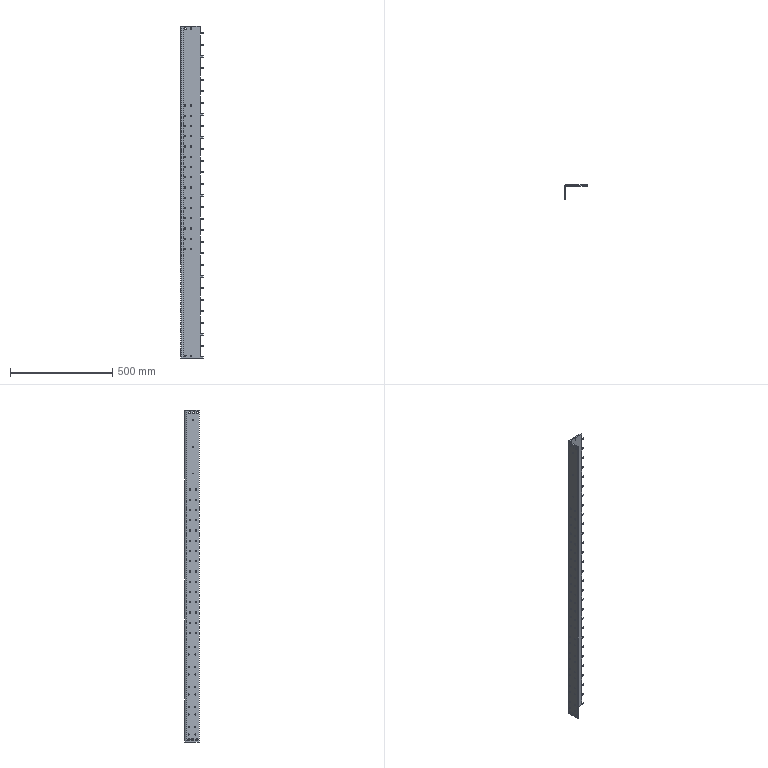Part | SolidWorks | features HoleWzd 8, Extrusion 1, Fillet 1, ICE 1, LPattern 1 | 1 solid | 335 faces | box 110 x 70 x 1620 mm | volume 1292912 mm3 | cylinder 193 | plane 132 | cone 10 | commonest cylinder face diameters 6.8 x120 5.8 x59 4.2 x6 5.5 x6 16 x2